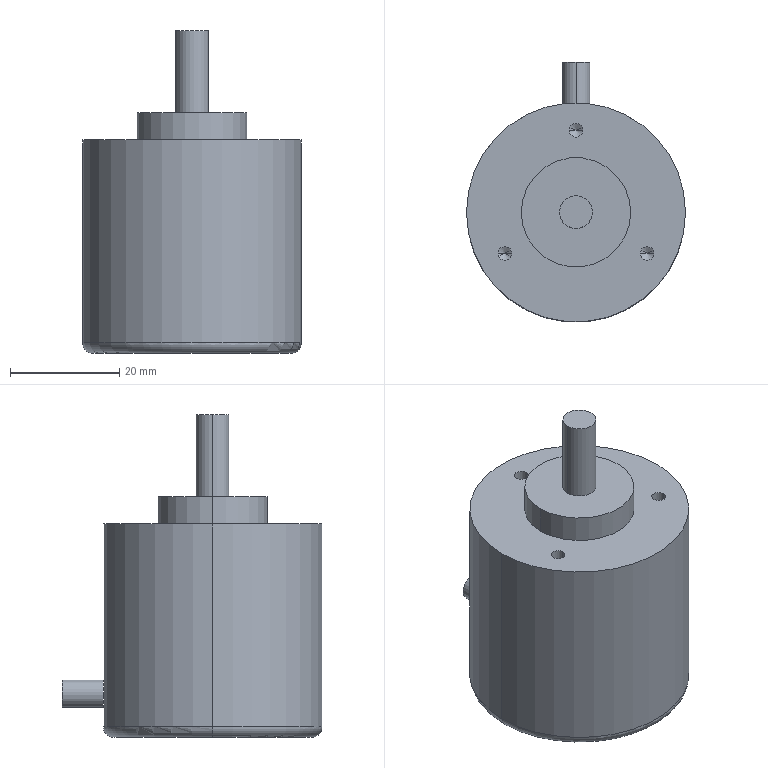Part | SolidWorks | features ICE 3, Extrusion 1, Fillet 1, HoleWzd 1 | 4 solids | 30 faces | box 40 x 47.5 x 59 mm | volume 50942 mm3 | cylinder 14 | plane 8 | cone 6 | torus 2 | commonest cylinder face diameters 2.5 x6 5 x2 6 x2 20 x2 40 x2
STEP:
#1=CARTESIAN_POINT('',(10.,0.,44.));
#2=VERTEX_POINT('',#1);
#3=CARTESIAN_POINT('',(-10.,0.,44.));
#4=VERTEX_POINT('',#3);
#5=CARTESIAN_POINT('',(0.,0.,44.));
#6=DIRECTION('',(0.,0.,1.));
#7=DIRECTION('',(1.,0.,0.));
#8=AXIS2_PLACEMENT_3D('',#5,#6,#7);
#9=CIRCLE('',#8,10.);
#10=EDGE_CURVE('',#2,#4,#9,.T.);
#11=ORIENTED_EDGE('',*,*,#10,.F.);
#12=CARTESIAN_POINT('',(10.,0.,39.));
#13=VERTEX_POINT('',#12);
#14=CARTESIAN_POINT('',(10.,0.,44.));
#15=DIRECTION('',(0.,0.,-1.));
#16=VECTOR('',#15,1000.);
#17=LINE('',#14,#16);
#18=EDGE_CURVE('',#2,#13,#17,.T.);
#19=ORIENTED_EDGE('',*,*,#18,.T.);
#20=CARTESIAN_POINT('',(-10.,0.,39.));
#21=VERTEX_POINT('',#20);
#22=CARTESIAN_POINT('',(0.,0.,39.));
#23=DIRECTION('',(0.,0.,1.));
#24=DIRECTION('',(1.,0.,0.));
#25=AXIS2_PLACEMENT_3D('',#22,#23,#24);
#26=CIRCLE('',#25,10.);
#27=EDGE_CURVE('',#13,#21,#26,.T.);
#28=ORIENTED_EDGE('',*,*,#27,.T.);
#29=CARTESIAN_POINT('',(-10.,0.,44.));
#30=DIRECTION('',(0.,0.,-1.));
#31=VECTOR('',#30,1000.);
#32=LINE('',#29,#31);
#33=EDGE_CURVE('',#4,#21,#32,.T.);
#34=ORIENTED_EDGE('',*,*,#33,.F.);
#35=EDGE_LOOP('',(#11,#19,#28,#34));
#36=FACE_OUTER_BOUND('',#35,.T.);
#37=CARTESIAN_POINT('',(0.,0.,44.));
#38=DIRECTION('',(0.,0.,-1.));
#39=DIRECTION('',(-1.,0.,0.));
#40=AXIS2_PLACEMENT_3D('',#37,#38,#39);
#41=CYLINDRICAL_SURFACE('',#40,10.);
#42=ADVANCED_FACE('',(#36),#41,.T.);
#43=ORIENTED_EDGE('',*,*,#18,.F.);
#44=CARTESIAN_POINT('',(0.,0.,44.));
#45=DIRECTION('',(0.,0.,1.));
#46=DIRECTION('',(1.,0.,0.));
#47=AXIS2_PLACEMENT_3D('',#44,#45,#46);
#48=CIRCLE('',#47,10.);
#49=EDGE_CURVE('',#4,#2,#48,.T.);
#50=ORIENTED_EDGE('',*,*,#49,.F.);
#51=ORIENTED_EDGE('',*,*,#33,.T.);
#52=CARTESIAN_POINT('',(0.,0.,39.));
#53=DIRECTION('',(0.,0.,1.));
#54=DIRECTION('',(1.,0.,0.));
#55=AXIS2_PLACEMENT_3D('',#52,#53,#54);
#56=CIRCLE('',#55,10.);
#57=EDGE_CURVE('',#21,#13,#56,.T.);
#58=ORIENTED_EDGE('',*,*,#57,.T.);
#59=EDGE_LOOP('',(#43,#50,#51,#58));
#60=FACE_OUTER_BOUND('',#59,.T.);
#61=CARTESIAN_POINT('',(0.,0.,44.));
#62=DIRECTION('',(0.,0.,-1.));
#63=DIRECTION('',(-1.,0.,0.));
#64=AXIS2_PLACEMENT_3D('',#61,#62,#63);
#65=CYLINDRICAL_SURFACE('',#64,10.);
#66=ADVANCED_FACE('',(#60),#65,.T.);
#67=ORIENTED_EDGE('',*,*,#49,.T.);
#68=ORIENTED_EDGE('',*,*,#10,.T.);
#69=EDGE_LOOP('',(#67,#68));
#70=FACE_OUTER_BOUND('',#69,.T.);
#71=CARTESIAN_POINT('',(0.,0.,44.));
#72=DIRECTION('',(0.,0.,1.));
#73=DIRECTION('',(1.,0.,0.));
#74=AXIS2_PLACEMENT_3D('',#71,#72,#73);
#75=PLANE('',#74);
#76=ADVANCED_FACE('',(#70),#75,.T.);
#77=ORIENTED_EDGE('',*,*,#57,.F.);
#78=ORIENTED_EDGE('',*,*,#27,.F.);
#79=EDGE_LOOP('',(#77,#78));
#80=FACE_OUTER_BOUND('',#79,.T.);
#81=CARTESIAN_POINT('',(0.,0.,39.));
#82=DIRECTION('',(0.,0.,1.));
#83=DIRECTION('',(1.,0.,0.));
#84=AXIS2_PLACEMENT_3D('',#81,#82,#83);
#85=PLANE('',#84);
#86=ADVANCED_FACE('',(#80),#85,.F.);
#87=CLOSED_SHELL('',(#42,#66,#76,#86));
#88=MANIFOLD_SOLID_BREP('',#87);
#89=CARTESIAN_POINT('',(3.,0.,59.));
#90=VERTEX_POINT('',#89);
#91=CARTESIAN_POINT('',(-3.,0.,59.));
#92=VERTEX_POINT('',#91);
#93=CARTESIAN_POINT('',(0.,0.,59.));
#94=DIRECTION('',(0.,0.,1.));
#95=DIRECTION('',(1.,0.,0.));
#96=AXIS2_PLACEMENT_3D('',#93,#94,#95);
#97=CIRCLE('',#96,3.);
#98=EDGE_CURVE('',#90,#92,#97,.T.);
#99=ORIENTED_EDGE('',*,*,#98,.F.);
#100=CARTESIAN_POINT('',(3.,0.,44.));
#101=VERTEX_POINT('',#100);
#102=CARTESIAN_POINT('',(3.,0.,59.));
#103=DIRECTION('',(0.,0.,-1.));
#104=VECTOR('',#103,1000.);
#105=LINE('',#102,#104);
#106=EDGE_CURVE('',#90,#101,#105,.T.);
#107=ORIENTED_EDGE('',*,*,#106,.T.);
#108=CARTESIAN_POINT('',(-3.,0.,44.));
#109=VERTEX_POINT('',#108);
#110=CARTESIAN_POINT('',(0.,0.,44.));
#111=DIRECTION('',(0.,0.,1.));
#112=DIRECTION('',(1.,0.,0.));
#113=AXIS2_PLACEMENT_3D('',#110,#111,#112);
#114=CIRCLE('',#113,3.);
#115=EDGE_CURVE('',#101,#109,#114,.T.);
#116=ORIENTED_EDGE('',*,*,#115,.T.);
#117=CARTESIAN_POINT('',(-3.,0.,59.));
#118=DIRECTION('',(0.,0.,-1.));
#119=VECTOR('',#118,1000.);
#120=LINE('',#117,#119);
#121=EDGE_CURVE('',#92,#109,#120,.T.);
#122=ORIENTED_EDGE('',*,*,#121,.F.);
#123=EDGE_LOOP('',(#99,#107,#116,#122));
#124=FACE_OUTER_BOUND('',#123,.T.);
#125=CARTESIAN_POINT('',(0.,0.,59.));
#126=DIRECTION('',(0.,0.,-1.));
#127=DIRECTION('',(-1.,0.,0.));
#128=AXIS2_PLACEMENT_3D('',#125,#126,#127);
#129=CYLINDRICAL_SURFACE('',#128,3.);
#130=ADVANCED_FACE('',(#124),#129,.T.);
#131=ORIENTED_EDGE('',*,*,#106,.F.);
#132=CARTESIAN_POINT('',(0.,0.,59.));
#133=DIRECTION('',(0.,0.,1.));
#134=DIRECTION('',(1.,0.,0.));
#135=AXIS2_PLACEMENT_3D('',#132,#133,#134);
#136=CIRCLE('',#135,3.);
#137=EDGE_CURVE('',#92,#90,#136,.T.);
#138=ORIENTED_EDGE('',*,*,#137,.F.);
#139=ORIENTED_EDGE('',*,*,#121,.T.);
#140=CARTESIAN_POINT('',(0.,0.,44.));
#141=DIRECTION('',(0.,0.,1.));
#142=DIRECTION('',(1.,0.,0.));
#143=AXIS2_PLACEMENT_3D('',#140,#141,#142);
#144=CIRCLE('',#143,3.);
#145=EDGE_CURVE('',#109,#101,#144,.T.);
#146=ORIENTED_EDGE('',*,*,#145,.T.);
#147=EDGE_LOOP('',(#131,#138,#139,#146));
#148=FACE_OUTER_BOUND('',#147,.T.);
#149=CARTESIAN_POINT('',(0.,0.,59.));
#150=DIRECTION('',(0.,0.,-1.));
#151=DIRECTION('',(-1.,0.,0.));
#152=AXIS2_PLACEMENT_3D('',#149,#150,#151);
#153=CYLINDRICAL_SURFACE('',#152,3.);
#154=ADVANCED_FACE('',(#148),#153,.T.);
#155=ORIENTED_EDGE('',*,*,#137,.T.);
#156=ORIENTED_EDGE('',*,*,#98,.T.);
#157=EDGE_LOOP('',(#155,#156));
#158=FACE_OUTER_BOUND('',#157,.T.);
#159=CARTESIAN_POINT('',(0.,0.,59.));
#160=DIRECTION('',(0.,0.,1.));
#161=DIRECTION('',(1.,0.,0.));
#162=AXIS2_PLACEMENT_3D('',#159,#160,#161);
#163=PLANE('',#162);
#164=ADVANCED_FACE('',(#158),#163,.T.);
#165=ORIENTED_EDGE('',*,*,#145,.F.);
#166=ORIENTED_EDGE('',*,*,#115,.F.);
#167=EDGE_LOOP('',(#165,#166));
#168=FACE_OUTER_BOUND('',#167,.T.);
#169=CARTESIAN_POINT('',(0.,0.,44.));
#170=DIRECTION('',(0.,0.,1.));
#171=DIRECTION('',(1.,0.,0.));
#172=AXIS2_PLACEMENT_3D('',#169,#170,#171);
#173=PLANE('',#172);
#174=ADVANCED_FACE('',(#168),#173,.F.);
#175=CLOSED_SHELL('',(#130,#154,#164,#174));
#176=MANIFOLD_SOLID_BREP('',#175);
#177=CARTESIAN_POINT('',(-18.,0.,0.));
#178=VERTEX_POINT('',#177);
#179=CARTESIAN_POINT('',(18.,0.,0.));
#180=VERTEX_POINT('',#179);
#181=CARTESIAN_POINT('',(0.,0.,0.));
#182=DIRECTION('',(0.,0.,-1.));
#183=DIRECTION('',(1.,0.,0.));
#184=AXIS2_PLACEMENT_3D('',#181,#182,#183);
#185=CIRCLE('',#184,18.);
#186=EDGE_CURVE('',#178,#180,#185,.T.);
#187=ORIENTED_EDGE('',*,*,#186,.F.);
#188=CARTESIAN_POINT('',(-20.,0.,2.));
#189=VERTEX_POINT('',#188);
#190=CARTESIAN_POINT('',(-18.,0.,2.));
#191=DIRECTION('',(0.,1.,0.));
#192=DIRECTION('',(-1.,0.,0.));
#193=AXIS2_PLACEMENT_3D('',#190,#191,#192);
#194=CIRCLE('',#193,2.);
#195=EDGE_CURVE('',#178,#189,#194,.T.);
#196=ORIENTED_EDGE('',*,*,#195,.T.);
#197=CARTESIAN_POINT('',(20.,0.,2.));
#198=VERTEX_POINT('',#197);
#199=CARTESIAN_POINT('',(0.,0.,2.));
#200=DIRECTION('',(0.,0.,1.));
#201=DIRECTION('',(1.,0.,0.));
#202=AXIS2_PLACEMENT_3D('',#199,#200,#201);
#203=CIRCLE('',#202,20.);
#204=EDGE_CURVE('',#198,#189,#203,.T.);
#205=ORIENTED_EDGE('',*,*,#204,.F.);
#206=CARTESIAN_POINT('',(18.,0.,2.));
#207=DIRECTION('',(0.,-1.,0.));
#208=DIRECTION('',(0.,0.,-1.));
#209=AXIS2_PLACEMENT_3D('',#206,#207,#208);
#210=CIRCLE('',#209,2.);
#211=EDGE_CURVE('',#180,#198,#210,.T.);
#212=ORIENTED_EDGE('',*,*,#211,.F.);
#213=EDGE_LOOP('',(#187,#196,#205,#212));
#214=FACE_OUTER_BOUND('',#213,.T.);
#215=CARTESIAN_POINT('',(0.,0.,2.));
#216=DIRECTION('',(0.,0.,1.));
#217=DIRECTION('',(1.,0.,0.));
#218=AXIS2_PLACEMENT_3D('',#215,#216,#217);
#219=TOROIDAL_SURFACE('',#218,18.,2.);
#220=ADVANCED_FACE('',(#214),#219,.T.);
#221=CARTESIAN_POINT('',(-1.25,15.,32.251));
#222=VERTEX_POINT('',#221);
#223=CARTESIAN_POINT('',(1.25,15.,32.251));
#224=VERTEX_POINT('',#223);
#225=CARTESIAN_POINT('',(0.,15.,32.251));
#226=DIRECTION('',(0.,0.,1.));
#227=DIRECTION('',(1.,0.,0.));
#228=AXIS2_PLACEMENT_3D('',#225,#226,#227);
#229=CIRCLE('',#228,1.25);
#230=EDGE_CURVE('',#222,#224,#229,.T.);
#231=ORIENTED_EDGE('',*,*,#230,.F.);
#232=CARTESIAN_POINT('',(-1.25,15.,39.));
#233=VERTEX_POINT('',#232);
#234=CARTESIAN_POINT('',(-1.25,15.,39.));
#235=DIRECTION('',(0.,0.,1.));
#236=VECTOR('',#235,1000.);
#237=LINE('',#234,#236);
#238=EDGE_CURVE('',#222,#233,#237,.T.);
#239=ORIENTED_EDGE('',*,*,#238,.T.);
#240=CARTESIAN_POINT('',(1.25,15.,39.));
#241=VERTEX_POINT('',#240);
#242=CARTESIAN_POINT('',(0.,15.,39.));
#243=DIRECTION('',(0.,0.,1.));
#244=DIRECTION('',(1.,0.,0.));
#245=AXIS2_PLACEMENT_3D('',#242,#243,#244);
#246=CIRCLE('',#245,1.25);
#247=EDGE_CURVE('',#233,#241,#246,.T.);
#248=ORIENTED_EDGE('',*,*,#247,.T.);
#249=CARTESIAN_POINT('',(1.25,15.,39.));
#250=DIRECTION('',(0.,0.,1.));
#251=VECTOR('',#250,1000.);
#252=LINE('',#249,#251);
#253=EDGE_CURVE('',#224,#241,#252,.T.);
#254=ORIENTED_EDGE('',*,*,#253,.F.);
#255=EDGE_LOOP('',(#231,#239,#248,#254));
#256=FACE_OUTER_BOUND('',#255,.T.);
#257=CARTESIAN_POINT('',(0.,15.,39.));
#258=DIRECTION('',(0.,0.,1.));
#259=DIRECTION('',(1.,0.,0.));
#260=AXIS2_PLACEMENT_3D('',#257,#258,#259);
#261=CYLINDRICAL_SURFACE('',#260,1.25);
#262=ADVANCED_FACE('',(#256),#261,.F.);
#263=CARTESIAN_POINT('',(0.,15.,31.5));
#264=VERTEX_POINT('',#263);
#265=CARTESIAN_POINT('',(1.25,15.,32.251));
#266=DIRECTION('',(0.8572,0.,0.515));
#267=VECTOR('',#266,1000.);
#268=LINE('',#265,#267);
#269=EDGE_CURVE('',#264,#224,#268,.T.);
#270=ORIENTED_EDGE('',*,*,#269,.F.);
#271=CARTESIAN_POINT('',(-1.25,15.,32.251));
#272=DIRECTION('',(-0.8572,0.,0.515));
#273=VECTOR('',#272,1000.);
#274=LINE('',#271,#273);
#275=EDGE_CURVE('',#264,#222,#274,.T.);
#276=ORIENTED_EDGE('',*,*,#275,.T.);
#277=ORIENTED_EDGE('',*,*,#230,.T.);
#278=EDGE_LOOP('',(#270,#276,#277));
#279=FACE_OUTER_BOUND('',#278,.T.);
#280=CARTESIAN_POINT('',(0.,15.,32.251));
#281=DIRECTION('',(0.,0.,1.));
#282=DIRECTION('',(1.,0.,0.));
#283=AXIS2_PLACEMENT_3D('',#280,#281,#282);
#284=CONICAL_SURFACE('',#283,1.25,1.03);
#285=ADVANCED_FACE('',(#279),#284,.F.);
#286=CARTESIAN_POINT('',(-14.24,-7.5,32.251));
#287=VERTEX_POINT('',#286);
#288=CARTESIAN_POINT('',(-11.74,-7.5,32.251));
#289=VERTEX_POINT('',#288);
#290=CARTESIAN_POINT('',(-12.99,-7.5,32.251));
#291=DIRECTION('',(0.,0.,1.));
#292=DIRECTION('',(1.,0.,0.));
#293=AXIS2_PLACEMENT_3D('',#290,#291,#292);
#294=CIRCLE('',#293,1.25);
#295=EDGE_CURVE('',#287,#289,#294,.T.);
#296=ORIENTED_EDGE('',*,*,#295,.F.);
#297=CARTESIAN_POINT('',(-14.24,-7.5,39.));
#298=VERTEX_POINT('',#297);
#299=CARTESIAN_POINT('',(-14.24,-7.5,39.));
#300=DIRECTION('',(0.,0.,1.));
#301=VECTOR('',#300,1000.);
#302=LINE('',#299,#301);
#303=EDGE_CURVE('',#287,#298,#302,.T.);
#304=ORIENTED_EDGE('',*,*,#303,.T.);
#305=CARTESIAN_POINT('',(-11.74,-7.5,39.));
#306=VERTEX_POINT('',#305);
#307=CARTESIAN_POINT('',(-12.99,-7.5,39.));
#308=DIRECTION('',(0.,0.,1.));
#309=DIRECTION('',(1.,0.,0.));
#310=AXIS2_PLACEMENT_3D('',#307,#308,#309);
#311=CIRCLE('',#310,1.25);
#312=EDGE_CURVE('',#298,#306,#311,.T.);
#313=ORIENTED_EDGE('',*,*,#312,.T.);
#314=CARTESIAN_POINT('',(-11.74,-7.5,39.));
#315=DIRECTION('',(0.,0.,1.));
#316=VECTOR('',#315,1000.);
#317=LINE('',#314,#316);
#318=EDGE_CURVE('',#289,#306,#317,.T.);
#319=ORIENTED_EDGE('',*,*,#318,.F.);
#320=EDGE_LOOP('',(#296,#304,#313,#319));
#321=FACE_OUTER_BOUND('',#320,.T.);
#322=CARTESIAN_POINT('',(-12.99,-7.5,39.));
#323=DIRECTION('',(0.,0.,1.));
#324=DIRECTION('',(1.,0.,0.));
#325=AXIS2_PLACEMENT_3D('',#322,#323,#324);
#326=CYLINDRICAL_SURFACE('',#325,1.25);
#327=ADVANCED_FACE('',(#321),#326,.F.);
#328=CARTESIAN_POINT('',(-12.99,-7.5,31.5));
#329=VERTEX_POINT('',#328);
#330=CARTESIAN_POINT('',(-11.74,-7.5,32.251));
#331=DIRECTION('',(0.8572,0.,0.515));
#332=VECTOR('',#331,1000.);
#333=LINE('',#330,#332);
#334=EDGE_CURVE('',#329,#289,#333,.T.);
#335=ORIENTED_EDGE('',*,*,#334,.F.);
#336=CARTESIAN_POINT('',(-14.24,-7.5,32.251));
#337=DIRECTION('',(-0.8572,0.,0.515));
#338=VECTOR('',#337,1000.);
#339=LINE('',#336,#338);
#340=EDGE_CURVE('',#329,#287,#339,.T.);
#341=ORIENTED_EDGE('',*,*,#340,.T.);
#342=ORIENTED_EDGE('',*,*,#295,.T.);
#343=EDGE_LOOP('',(#335,#341,#342));
#344=FACE_OUTER_BOUND('',#343,.T.);
#345=CARTESIAN_POINT('',(-12.99,-7.5,32.251));
#346=DIRECTION('',(0.,0.,1.));
#347=DIRECTION('',(1.,0.,0.));
#348=AXIS2_PLACEMENT_3D('',#345,#346,#347);
#349=CONICAL_SURFACE('',#348,1.25,1.03);
#350=ADVANCED_FACE('',(#344),#349,.F.);
#351=CARTESIAN_POINT('',(11.74,-7.5,32.251));
#352=VERTEX_POINT('',#351);
#353=CARTESIAN_POINT('',(14.24,-7.5,32.251));
#354=VERTEX_POINT('',#353);
#355=CARTESIAN_POINT('',(12.99,-7.5,32.251));
#356=DIRECTION('',(0.,0.,1.));
#357=DIRECTION('',(1.,0.,0.));
#358=AXIS2_PLACEMENT_3D('',#355,#356,#357);
#359=CIRCLE('',#358,1.25);
#360=EDGE_CURVE('',#352,#354,#359,.T.);
#361=ORIENTED_EDGE('',*,*,#360,.F.);
#362=CARTESIAN_POINT('',(11.74,-7.5,39.));
#363=VERTEX_POINT('',#362);
#364=CARTESIAN_POINT('',(11.74,-7.5,39.));
#365=DIRECTION('',(0.,0.,1.));
#366=VECTOR('',#365,1000.);
#367=LINE('',#364,#366);
#368=EDGE_CURVE('',#352,#363,#367,.T.);
#369=ORIENTED_EDGE('',*,*,#368,.T.);
#370=CARTESIAN_POINT('',(14.24,-7.5,39.));
#371=VERTEX_POINT('',#370);
#372=CARTESIAN_POINT('',(12.99,-7.5,39.));
#373=DIRECTION('',(0.,0.,1.));
#374=DIRECTION('',(1.,0.,0.));
#375=AXIS2_PLACEMENT_3D('',#372,#373,#374);
#376=CIRCLE('',#375,1.25);
#377=EDGE_CURVE('',#363,#371,#376,.T.);
#378=ORIENTED_EDGE('',*,*,#377,.T.);
#379=CARTESIAN_POINT('',(14.24,-7.5,39.));
#380=DIRECTION('',(0.,0.,1.));
#381=VECTOR('',#380,1000.);
#382=LINE('',#379,#381);
#383=EDGE_CURVE('',#354,#371,#382,.T.);
#384=ORIENTED_EDGE('',*,*,#383,.F.);
#385=EDGE_LOOP('',(#361,#369,#378,#384));
#386=FACE_OUTER_BOUND('',#385,.T.);
#387=CARTESIAN_POINT('',(12.99,-7.5,39.));
#388=DIRECTION('',(0.,0.,1.));
#389=DIRECTION('',(1.,0.,0.));
#390=AXIS2_PLACEMENT_3D('',#387,#388,#389);
#391=CYLINDRICAL_SURFACE('',#390,1.25);
#392=ADVANCED_FACE('',(#386),#391,.F.);
#393=CARTESIAN_POINT('',(12.99,-7.5,31.5));
#394=VERTEX_POINT('',#393);
#395=CARTESIAN_POINT('',(14.24,-7.5,32.251));
#396=DIRECTION('',(0.8572,0.,0.515));
#397=VECTOR('',#396,1000.);
#398=LINE('',#395,#397);
#399=EDGE_CURVE('',#394,#354,#398,.T.);
#400=ORIENTED_EDGE('',*,*,#399,.F.);
#401=CARTESIAN_POINT('',(11.74,-7.5,32.251));
#402=DIRECTION('',(-0.8572,0.,0.515));
#403=VECTOR('',#402,1000.);
#404=LINE('',#401,#403);
#405=EDGE_CURVE('',#394,#352,#404,.T.);
#406=ORIENTED_EDGE('',*,*,#405,.T.);
#407=ORIENTED_EDGE('',*,*,#360,.T.);
#408=EDGE_LOOP('',(#400,#406,#407));
#409=FACE_OUTER_BOUND('',#408,.T.);
#410=CARTESIAN_POINT('',(12.99,-7.5,32.251));
#411=DIRECTION('',(0.,0.,1.));
#412=DIRECTION('',(1.,0.,0.));
#413=AXIS2_PLACEMENT_3D('',#410,#411,#412);
#414=CONICAL_SURFACE('',#413,1.25,1.03);
#415=ADVANCED_FACE('',(#409),#414,.F.);
#416=CARTESIAN_POINT('',(20.,0.,39.));
#417=VERTEX_POINT('',#416);
#418=CARTESIAN_POINT('',(-20.,0.,39.));
#419=VERTEX_POINT('',#418);
#420=CARTESIAN_POINT('',(0.,0.,39.));
#421=DIRECTION('',(0.,0.,1.));
#422=DIRECTION('',(1.,0.,0.));
#423=AXIS2_PLACEMENT_3D('',#420,#421,#422);
#424=CIRCLE('',#423,20.);
#425=EDGE_CURVE('',#417,#419,#424,.T.);
#426=ORIENTED_EDGE('',*,*,#425,.F.);
#427=CARTESIAN_POINT('',(20.,0.,39.));
#428=DIRECTION('',(0.,0.,-1.));
#429=VECTOR('',#428,1000.);
#430=LINE('',#427,#429);
#431=EDGE_CURVE('',#417,#198,#430,.T.);
#432=ORIENTED_EDGE('',*,*,#431,.T.);
#433=ORIENTED_EDGE('',*,*,#204,.T.);
#434=CARTESIAN_POINT('',(-20.,0.,39.));
#435=DIRECTION('',(0.,0.,-1.));
#436=VECTOR('',#435,1000.);
#437=LINE('',#434,#436);
#438=EDGE_CURVE('',#419,#189,#437,.T.);
#439=ORIENTED_EDGE('',*,*,#438,.F.);
#440=EDGE_LOOP('',(#426,#432,#433,#439));
#441=FACE_OUTER_BOUND('',#440,.T.);
#442=CARTESIAN_POINT('',(0.,0.,39.));
#443=DIRECTION('',(0.,0.,-1.));
#444=DIRECTION('',(-1.,0.,0.));
#445=AXIS2_PLACEMENT_3D('',#442,#443,#444);
#446=CYLINDRICAL_SURFACE('',#445,20.);
#447=ADVANCED_FACE('',(#441),#446,.T.);
#448=ORIENTED_EDGE('',*,*,#431,.F.);
#449=CARTESIAN_POINT('',(0.,0.,39.));
#450=DIRECTION('',(0.,0.,1.));
#451=DIRECTION('',(1.,0.,0.));
#452=AXIS2_PLACEMENT_3D('',#449,#450,#451);
#453=CIRCLE('',#452,20.);
#454=EDGE_CURVE('',#419,#417,#453,.T.);
#455=ORIENTED_EDGE('',*,*,#454,.F.);
#456=ORIENTED_EDGE('',*,*,#438,.T.);
#457=CARTESIAN_POINT('',(0.,0.,2.));
#458=DIRECTION('',(0.,0.,1.));
#459=DIRECTION('',(1.,0.,0.));
#460=AXIS2_PLACEMENT_3D('',#457,#458,#459);
#461=CIRCLE('',#460,20.);
#462=EDGE_CURVE('',#189,#198,#461,.T.);
#463=ORIENTED_EDGE('',*,*,#462,.T.);
#464=EDGE_LOOP('',(#448,#455,#456,#463));
#465=FACE_OUTER_BOUND('',#464,.T.);
#466=CARTESIAN_POINT('',(0.,0.,39.));
#467=DIRECTION('',(0.,0.,-1.));
#468=DIRECTION('',(-1.,0.,0.));
#469=AXIS2_PLACEMENT_3D('',#466,#467,#468);
#470=CYLINDRICAL_SURFACE('',#469,20.);
#471=ADVANCED_FACE('',(#465),#470,.T.);
#472=CARTESIAN_POINT('',(0.,15.,39.));
#473=DIRECTION('',(0.,0.,1.));
#474=DIRECTION('',(1.,0.,0.));
#475=AXIS2_PLACEMENT_3D('',#472,#473,#474);
#476=CIRCLE('',#475,1.25);
#477=EDGE_CURVE('',#241,#233,#476,.T.);
#478=ORIENTED_EDGE('',*,*,#477,.F.);
#479=ORIENTED_EDGE('',*,*,#247,.F.);
#480=EDGE_LOOP('',(#478,#479));
#481=FACE_BOUND('',#480,.T.);
#482=CARTESIAN_POINT('',(-12.99,-7.5,39.));
#483=DIRECTION('',(0.,0.,1.));
#484=DIRECTION('',(1.,0.,0.));
#485=AXIS2_PLACEMENT_3D('',#482,#483,#484);
#486=CIRCLE('',#485,1.25);
#487=EDGE_CURVE('',#306,#298,#486,.T.);
#488=ORIENTED_EDGE('',*,*,#487,.F.);
#489=ORIENTED_EDGE('',*,*,#312,.F.);
#490=EDGE_LOOP('',(#488,#489));
#491=FACE_BOUND('',#490,.T.);
#492=CARTESIAN_POINT('',(12.99,-7.5,39.));
#493=DIRECTION('',(0.,0.,1.));
#494=DIRECTION('',(1.,0.,0.));
#495=AXIS2_PLACEMENT_3D('',#492,#493,#494);
#496=CIRCLE('',#495,1.25);
#497=EDGE_CURVE('',#371,#363,#496,.T.);
#498=ORIENTED_EDGE('',*,*,#497,.F.);
#499=ORIENTED_EDGE('',*,*,#377,.F.);
#500=EDGE_LOOP('',(#498,#499));
#501=FACE_BOUND('',#500,.T.);
#502=ORIENTED_EDGE('',*,*,#454,.T.);
#503=ORIENTED_EDGE('',*,*,#425,.T.);
#504=EDGE_LOOP('',(#502,#503));
#505=FACE_OUTER_BOUND('',#504,.T.);
#506=CARTESIAN_POINT('',(0.,0.,39.));
#507=DIRECTION('',(0.,0.,1.));
#508=DIRECTION('',(1.,0.,0.));
#509=AXIS2_PLACEMENT_3D('',#506,#507,#508);
#510=PLANE('',#509);
#511=ADVANCED_FACE('',(#481,#491,#501,#505),#510,.T.);
#512=CARTESIAN_POINT('',(0.,0.,0.));
#513=DIRECTION('',(0.,0.,-1.));
#514=DIRECTION('',(1.,0.,0.));
#515=AXIS2_PLACEMENT_3D('',#512,#513,#514);
#516=CIRCLE('',#515,18.);
#517=EDGE_CURVE('',#180,#178,#516,.T.);
#518=ORIENTED_EDGE('',*,*,#517,.T.);
#519=ORIENTED_EDGE('',*,*,#186,.T.);
#520=EDGE_LOOP('',(#518,#519));
#521=FACE_OUTER_BOUND('',#520,.T.);
#522=CARTESIAN_POINT('',(0.,0.,0.));
#523=DIRECTION('',(0.,0.,1.));
#524=DIRECTION('',(1.,0.,0.));
#525=AXIS2_PLACEMENT_3D('',#522,#523,#524);
#526=PLANE('',#525);
#527=ADVANCED_FACE('',(#521),#526,.F.);
#528=ORIENTED_EDGE('',*,*,#405,.F.);
#529=ORIENTED_EDGE('',*,*,#399,.T.);
#530=CARTESIAN_POINT('',(12.99,-7.5,32.251));
#531=DIRECTION('',(0.,0.,1.));
#532=DIRECTION('',(1.,0.,0.));
#533=AXIS2_PLACEMENT_3D('',#530,#531,#532);
#534=CIRCLE('',#533,1.25);
#535=EDGE_CURVE('',#354,#352,#534,.T.);
#536=ORIENTED_EDGE('',*,*,#535,.T.);
#537=EDGE_LOOP('',(#528,#529,#536));
#538=FACE_OUTER_BOUND('',#537,.T.);
#539=CARTESIAN_POINT('',(12.99,-7.5,32.251));
#540=DIRECTION('',(0.,0.,1.));
#541=DIRECTION('',(1.,0.,0.));
#542=AXIS2_PLACEMENT_3D('',#539,#540,#541);
#543=CONICAL_SURFACE('',#542,1.25,1.03);
#544=ADVANCED_FACE('',(#538),#543,.F.);
#545=ORIENTED_EDGE('',*,*,#368,.F.);
#546=ORIENTED_EDGE('',*,*,#535,.F.);
#547=ORIENTED_EDGE('',*,*,#383,.T.);
#548=ORIENTED_EDGE('',*,*,#497,.T.);
#549=EDGE_LOOP('',(#545,#546,#547,#548));
#550=FACE_OUTER_BOUND('',#549,.T.);
#551=CARTESIAN_POINT('',(12.99,-7.5,39.));
#552=DIRECTION('',(0.,0.,1.));
#553=DIRECTION('',(1.,0.,0.));
#554=AXIS2_PLACEMENT_3D('',#551,#552,#553);
#555=CYLINDRICAL_SURFACE('',#554,1.25);
#556=ADVANCED_FACE('',(#550),#555,.F.);
#557=ORIENTED_EDGE('',*,*,#340,.F.);
#558=ORIENTED_EDGE('',*,*,#334,.T.);
#559=CARTESIAN_POINT('',(-12.99,-7.5,32.251));
#560=DIRECTION('',(0.,0.,1.));
#561=DIRECTION('',(1.,0.,0.));
#562=AXIS2_PLACEMENT_3D('',#559,#560,#561);
#563=CIRCLE('',#562,1.25);
#564=EDGE_CURVE('',#289,#287,#563,.T.);
#565=ORIENTED_EDGE('',*,*,#564,.T.);
#566=EDGE_LOOP('',(#557,#558,#565));
#567=FACE_OUTER_BOUND('',#566,.T.);
#568=CARTESIAN_POINT('',(-12.99,-7.5,32.251));
#569=DIRECTION('',(0.,0.,1.));
#570=DIRECTION('',(1.,0.,0.));
#571=AXIS2_PLACEMENT_3D('',#568,#569,#570);
#572=CONICAL_SURFACE('',#571,1.25,1.03);
#573=ADVANCED_FACE('',(#567),#572,.F.);
#574=ORIENTED_EDGE('',*,*,#303,.F.);
#575=ORIENTED_EDGE('',*,*,#564,.F.);
#576=ORIENTED_EDGE('',*,*,#318,.T.);
#577=ORIENTED_EDGE('',*,*,#487,.T.);
#578=EDGE_LOOP('',(#574,#575,#576,#577));
#579=FACE_OUTER_BOUND('',#578,.T.);
#580=CARTESIAN_POINT('',(-12.99,-7.5,39.));
#581=DIRECTION('',(0.,0.,1.));
#582=DIRECTION('',(1.,0.,0.));
#583=AXIS2_PLACEMENT_3D('',#580,#581,#582);
#584=CYLINDRICAL_SURFACE('',#583,1.25);
#585=ADVANCED_FACE('',(#579),#584,.F.);
#586=ORIENTED_EDGE('',*,*,#275,.F.);
#587=ORIENTED_EDGE('',*,*,#269,.T.);
#588=CARTESIAN_POINT('',(0.,15.,32.251));
#589=DIRECTION('',(0.,0.,1.));
#590=DIRECTION('',(1.,0.,0.));
#591=AXIS2_PLACEMENT_3D('',#588,#589,#590);
#592=CIRCLE('',#591,1.25);
#593=EDGE_CURVE('',#224,#222,#592,.T.);
#594=ORIENTED_EDGE('',*,*,#593,.T.);
#595=EDGE_LOOP('',(#586,#587,#594));
#596=FACE_OUTER_BOUND('',#595,.T.);
#597=CARTESIAN_POINT('',(0.,15.,32.251));
#598=DIRECTION('',(0.,0.,1.));
#599=DIRECTION('',(1.,0.,0.));
#600=AXIS2_PLACEMENT_3D('',#597,#598,#599);
#601=CONICAL_SURFACE('',#600,1.25,1.03);
#602=ADVANCED_FACE('',(#596),#601,.F.);
#603=ORIENTED_EDGE('',*,*,#238,.F.);
#604=ORIENTED_EDGE('',*,*,#593,.F.);
#605=ORIENTED_EDGE('',*,*,#253,.T.);
#606=ORIENTED_EDGE('',*,*,#477,.T.);
#607=EDGE_LOOP('',(#603,#604,#605,#606));
#608=FACE_OUTER_BOUND('',#607,.T.);
#609=CARTESIAN_POINT('',(0.,15.,39.));
#610=DIRECTION('',(0.,0.,1.));
#611=DIRECTION('',(1.,0.,0.));
#612=AXIS2_PLACEMENT_3D('',#609,#610,#611);
#613=CYLINDRICAL_SURFACE('',#612,1.25);
#614=ADVANCED_FACE('',(#608),#613,.F.);
#615=ORIENTED_EDGE('',*,*,#195,.F.);
#616=ORIENTED_EDGE('',*,*,#517,.F.);
#617=ORIENTED_EDGE('',*,*,#211,.T.);
#618=ORIENTED_EDGE('',*,*,#462,.F.);
#619=EDGE_LOOP('',(#615,#616,#617,#618));
#620=FACE_OUTER_BOUND('',#619,.T.);
#621=CARTESIAN_POINT('',(0.,0.,2.));
#622=DIRECTION('',(0.,0.,1.));
#623=DIRECTION('',(1.,0.,0.));
#624=AXIS2_PLACEMENT_3D('',#621,#622,#623);
#625=TOROIDAL_SURFACE('',#624,18.,2.);
#626=ADVANCED_FACE('',(#620),#625,.T.);
#627=CLOSED_SHELL('',(#220,#262,#285,#327,#350,#392,#415,#447,#471,#511,#527,#544,#556,#573,#585,#602,#614,#626));
#628=MANIFOLD_SOLID_BREP('',#627);
#629=CARTESIAN_POINT('',(0.,27.5,10.5));
#630=VERTEX_POINT('',#629);
#631=CARTESIAN_POINT('',(0.,27.5,5.5));
#632=VERTEX_POINT('',#631);
#633=CARTESIAN_POINT('',(0.,27.5,8.));
#634=DIRECTION('',(0.,1.,0.));
#635=DIRECTION('',(0.,0.,1.));
#636=AXIS2_PLACEMENT_3D('',#633,#634,#635);
#637=CIRCLE('',#636,2.5);
#638=EDGE_CURVE('',#630,#632,#637,.T.);
#639=ORIENTED_EDGE('',*,*,#638,.F.);
#640=CARTESIAN_POINT('',(0.,20.,10.5));
#641=VERTEX_POINT('',#640);
#642=CARTESIAN_POINT('',(0.,27.5,10.5));
#643=DIRECTION('',(0.,-1.,0.));
#644=VECTOR('',#643,1000.);
#645=LINE('',#642,#644);
#646=EDGE_CURVE('',#630,#641,#645,.T.);
#647=ORIENTED_EDGE('',*,*,#646,.T.);
#648=CARTESIAN_POINT('',(0.,20.,5.5));
#649=VERTEX_POINT('',#648);
#650=CARTESIAN_POINT('',(0.,20.,8.));
#651=DIRECTION('',(0.,1.,0.));
#652=DIRECTION('',(0.,0.,1.));
#653=AXIS2_PLACEMENT_3D('',#650,#651,#652);
#654=CIRCLE('',#653,2.5);
#655=EDGE_CURVE('',#641,#649,#654,.T.);
#656=ORIENTED_EDGE('',*,*,#655,.T.);
#657=CARTESIAN_POINT('',(0.,27.5,5.5));
#658=DIRECTION('',(0.,-1.,0.));
#659=VECTOR('',#658,1000.);
#660=LINE('',#657,#659);
#661=EDGE_CURVE('',#632,#649,#660,.T.);
#662=ORIENTED_EDGE('',*,*,#661,.F.);
#663=EDGE_LOOP('',(#639,#647,#656,#662));
#664=FACE_OUTER_BOUND('',#663,.T.);
#665=CARTESIAN_POINT('',(0.,27.5,8.));
#666=DIRECTION('',(0.,-1.,0.));
#667=DIRECTION('',(0.,0.,-1.));
#668=AXIS2_PLACEMENT_3D('',#665,#666,#667);
#669=CYLINDRICAL_SURFACE('',#668,2.5);
#670=ADVANCED_FACE('',(#664),#669,.T.);
#671=ORIENTED_EDGE('',*,*,#646,.F.);
#672=CARTESIAN_POINT('',(0.,27.5,8.));
#673=DIRECTION('',(0.,1.,0.));
#674=DIRECTION('',(0.,0.,1.));
#675=AXIS2_PLACEMENT_3D('',#672,#673,#674);
#676=CIRCLE('',#675,2.5);
#677=EDGE_CURVE('',#632,#630,#676,.T.);
#678=ORIENTED_EDGE('',*,*,#677,.F.);
#679=ORIENTED_EDGE('',*,*,#661,.T.);
#680=CARTESIAN_POINT('',(0.,20.,8.));
#681=DIRECTION('',(0.,1.,0.));
#682=DIRECTION('',(0.,0.,1.));
#683=AXIS2_PLACEMENT_3D('',#680,#681,#682);
#684=CIRCLE('',#683,2.5);
#685=EDGE_CURVE('',#649,#641,#684,.T.);
#686=ORIENTED_EDGE('',*,*,#685,.T.);
#687=EDGE_LOOP('',(#671,#678,#679,#686));
#688=FACE_OUTER_BOUND('',#687,.T.);
#689=CARTESIAN_POINT('',(0.,27.5,8.));
#690=DIRECTION('',(0.,-1.,0.));
#691=DIRECTION('',(0.,0.,-1.));
#692=AXIS2_PLACEMENT_3D('',#689,#690,#691);
#693=CYLINDRICAL_SURFACE('',#692,2.5);
#694=ADVANCED_FACE('',(#688),#693,.T.);
#695=ORIENTED_EDGE('',*,*,#677,.T.);
#696=ORIENTED_EDGE('',*,*,#638,.T.);
#697=EDGE_LOOP('',(#695,#696));
#698=FACE_OUTER_BOUND('',#697,.T.);
#699=CARTESIAN_POINT('',(0.,27.5,8.));
#700=DIRECTION('',(0.,1.,0.));
#701=DIRECTION('',(0.,0.,1.));
#702=AXIS2_PLACEMENT_3D('',#699,#700,#701);
#703=PLANE('',#702);
#704=ADVANCED_FACE('',(#698),#703,.T.);
#705=ORIENTED_EDGE('',*,*,#685,.F.);
#706=ORIENTED_EDGE('',*,*,#655,.F.);
#707=EDGE_LOOP('',(#705,#706));
#708=FACE_OUTER_BOUND('',#707,.T.);
#709=CARTESIAN_POINT('',(0.,20.,8.));
#710=DIRECTION('',(0.,1.,0.));
#711=DIRECTION('',(0.,0.,1.));
#712=AXIS2_PLACEMENT_3D('',#709,#710,#711);
#713=PLANE('',#712);
#714=ADVANCED_FACE('',(#708),#713,.F.);
#715=CLOSED_SHELL('',(#670,#694,#704,#714));
#716=MANIFOLD_SOLID_BREP('',#715);
#717=CARTESIAN_POINT('',(0.,0.,0.));
#718=DIRECTION('',(0.,0.,1.));
#719=DIRECTION('',(1.,0.,0.));
#720=AXIS2_PLACEMENT_3D('',#717,#718,#719);
#721=(LENGTH_UNIT()NAMED_UNIT(*)SI_UNIT(.MILLI.,.METRE.));
#722=UNCERTAINTY_MEASURE_WITH_UNIT(LENGTH_MEASURE(0.00001),#721,'','');
#723=(NAMED_UNIT(*)PLANE_ANGLE_UNIT()SI_UNIT($,.RADIAN.));
#724=(NAMED_UNIT(*)SI_UNIT($,.STERADIAN.)SOLID_ANGLE_UNIT());
#725=(GEOMETRIC_REPRESENTATION_CONTEXT(3)GLOBAL_UNCERTAINTY_ASSIGNED_CONTEXT((#722))GLOBAL_UNIT_ASSIGNED_CONTEXT((#721,#723,#724))REPRESENTATION_CONTEXT('',''));
#726=ADVANCED_BREP_SHAPE_REPRESENTATION('',(#88,#176,#628,#716,#720),#725);